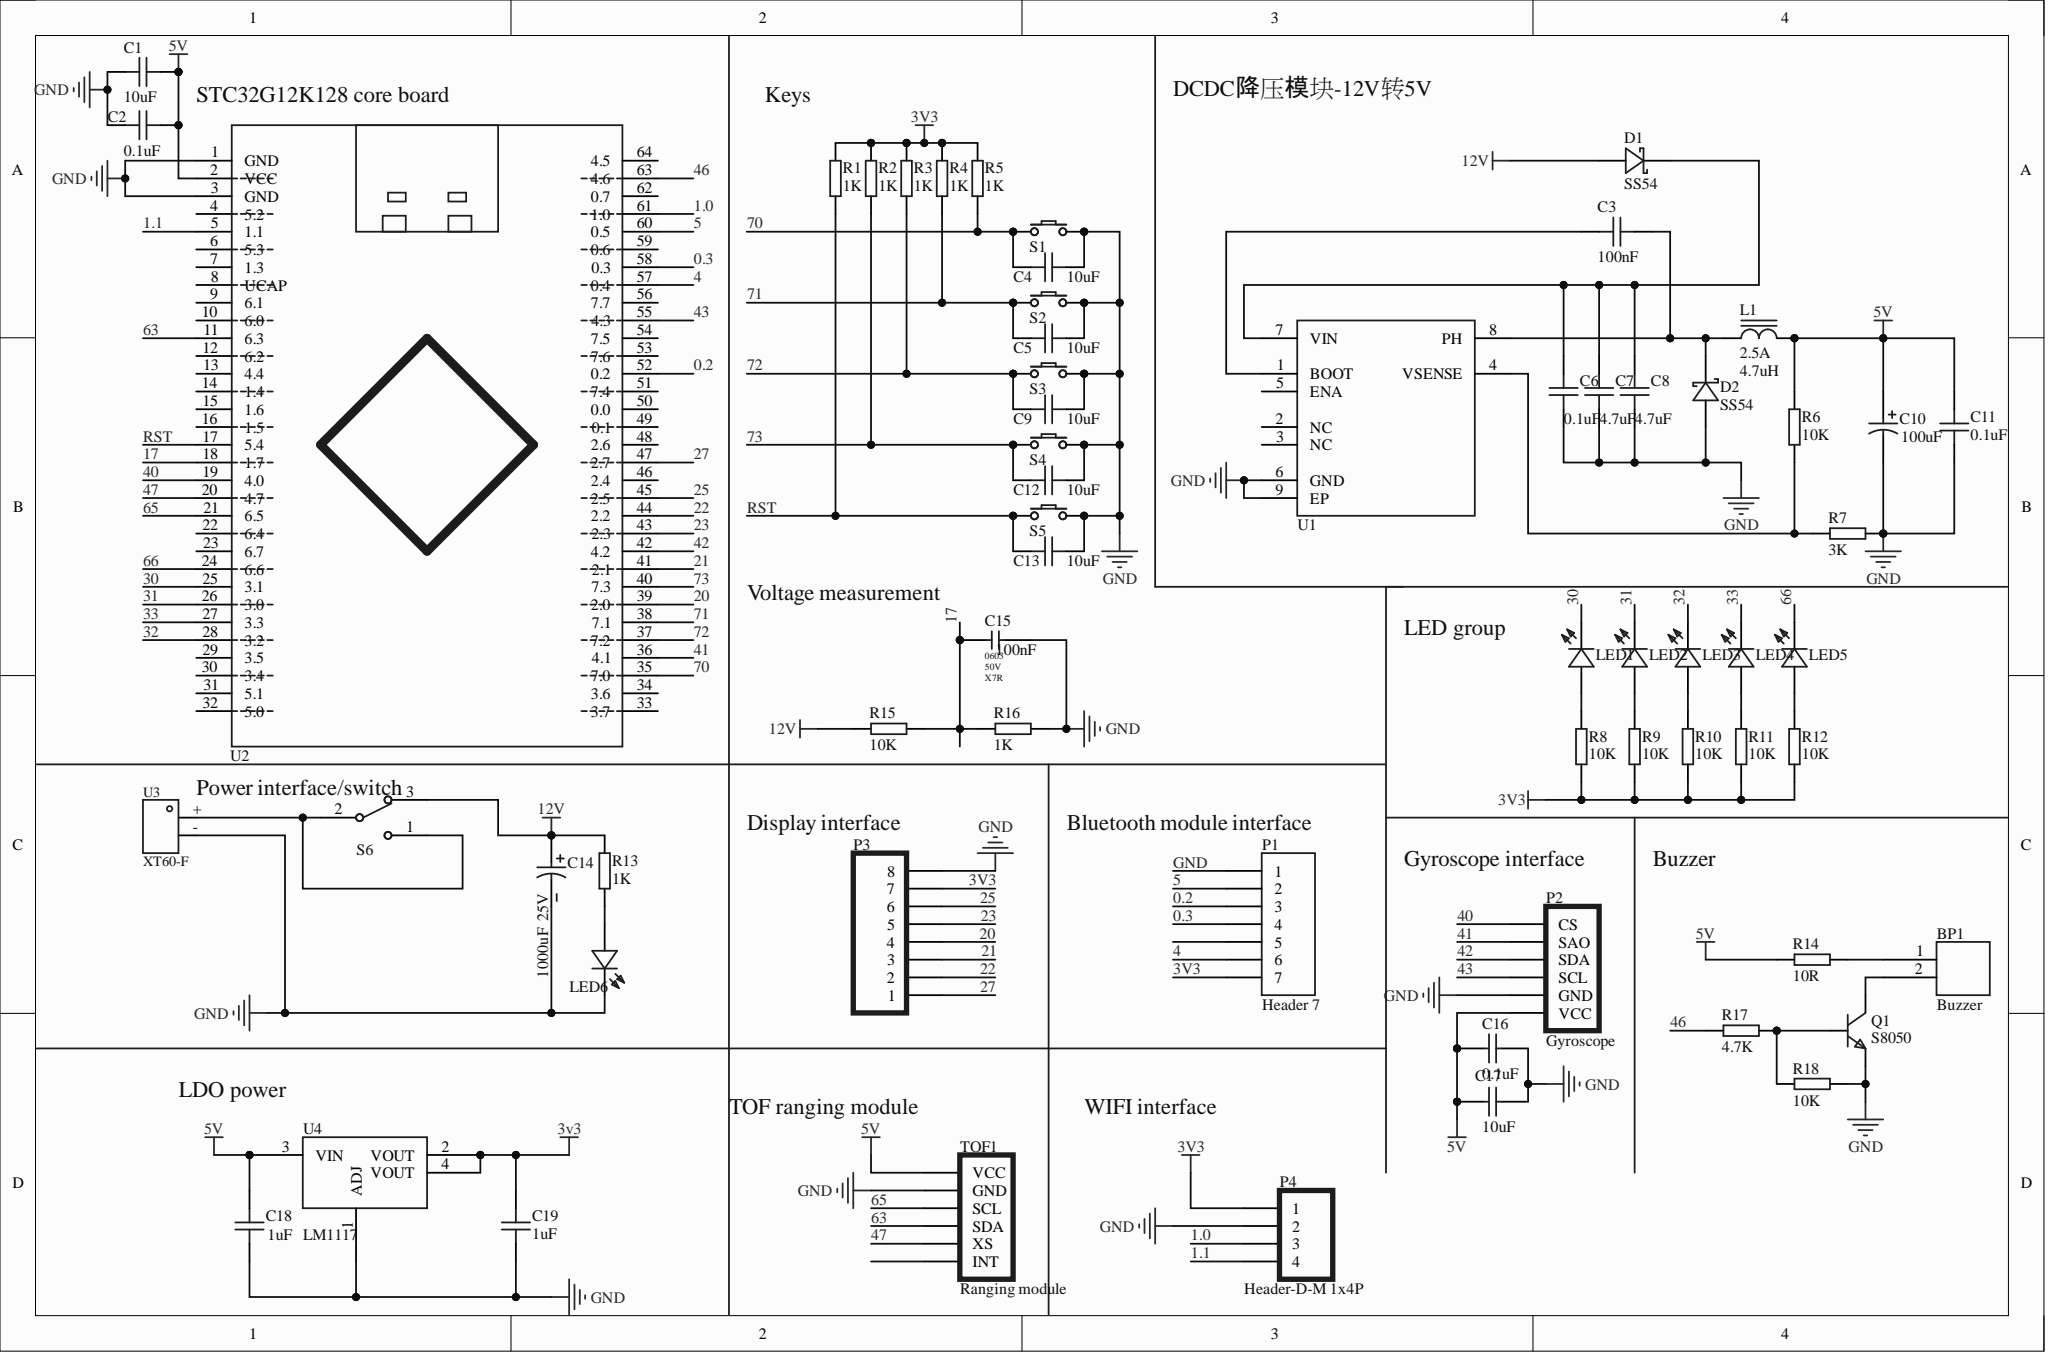Circuit board | Altium Designer | 63 parts | 49 nets
Bill of materials:
Comment,Description,Designator,Footprint,LibRef,Quantity
"Buzzer","","BP1","5*10fengmiqi","蜂鸣器","1"
"10uF","SMD capacitor","C1, C4, C5, C9, C12, C13","CAPC1608[0603]S-N","10uF","6"
"0.1uF","SMD capacitor","C2, C6, C11","CAPC1608[0603]S-N","0.1uF","3"
"100nF","SMD capacitor","C3","CAPC1608[0603]S-N","100nF","1"
"4.7uF","SMD capacitor","C7, C8","CAPC1608[0603]S-N","4.7uF","2"
"","Polarized Capacitor (Radial), SMD ceramic capacitor; MLCC; 0603(1608);, SMD capacitor","C10, C15, C16, C17","CAPC1608[0603]S-N","=Value+' '+Voltage, =Value +' '+ Voltage + ' ' + Type, =Value + ' ' + Tolerance +' '+ Voltage, =Value + ' ' + Tolerance +' '+ Voltage_1","4"
"1000uF  25V","Through-hole electrolytic capacitor","C14","CAPC1608[0603]S-N","1000uF  25V","1"
"1uF","SMD capacitor","C18, C19","CAPC1608[0603]S-N","1uF","2"
"SS54","SS54 Schottky diode","D1, D2","SOD-123-L","SS54","2"
"","Power inductor","L1","0402 TPC 4*4*2","=Value + ' ' + Imax","1"
"LED","SMD LED","LED1, LED2, LED3, LED4, LED5, LED6","LEDC1608(0603)","LED","6"
"Header 7","Header, 7-Pin","P1","HDR1X7","Header 7","1"
"Gyroscope","Header, 6-Pin","P2","HDR1X6","陀螺仪","1"
"Header  1X8","1X8","P3","HDR1X8","Header  1X8","1"
"Header-D-M 1x4P","1x4pin, through-hole, pin header","P4","HDR1X4","Header-D-M 1x4P","1"
"S8050","Discrete NPN Bipolar Transistor","Q1","SOT-23","S8050","1"
"1K","SMD resistor","R1, R2, R3, R4, R5, R13","RESC1608[0603]S-N","1K","6"
"10K","SMD resistor","R6, R8, R9, R10, R11, R12","RESC1608[0603]S-N","10K","6"
"3K","SMD resistor","R7","RESC1608[0603]S-N","3K","1"
"","SMD resistor","R14, R15, R16, R17, R18","RESC1608[0603]S-N","=Value+' '+Tolerance_2, =Value+' '+Tolerance_1, =Value+' '+Tolerance, =Value+' '+Tolerance_3","5"
"KEY","Keys","S1, S2, S3, S4, S5","anjiantiepiankaiguan","KEY","5"
"SW","SPDT switch","S6","SS12D10","SW","1"
"Ranging module","Header, 6-Pin","TOF1","HDR1X6","测距模块","1"
"TPS5450","5v regulator chip","U1","5450","TPS5450","1"
"STC32G12K128","STC32G12K128 core board","U2","STC16F40K128_CoreBoard","STC32G12K128","1"
"XT60-F","","U3","XT60","XT60-F","1"
"LM1117","3.3V regulator","U4","LM1117 - duplicate","LM1117","1"
Netlist (Protel format):
[
BP1
5*10fengmiqi
Buzzer



]
[
C1
CAPC1608[0603]S-N
10uF



]
[
C2
CAPC1608[0603]S-N
0.1uF



]
[
C3
CAPC1608[0603]S-N
100nF



]
[
C4
CAPC1608[0603]S-N
10uF



]
[
C5
CAPC1608[0603]S-N
10uF



]
[
C6
CAPC1608[0603]S-N
0.1uF



]
[
C7
CAPC1608[0603]S-N
4.7uF



]
[
C8
CAPC1608[0603]S-N
4.7uF



]
[
C9
CAPC1608[0603]S-N
10uF



]
[
C10
CAPC1608[0603]S-N




]
[
C11
CAPC1608[0603]S-N
0.1uF



]
[
C12
CAPC1608[0603]S-N
10uF



]
[
C13
CAPC1608[0603]S-N
10uF



]
[
C14
CAPC1608[0603]S-N
1000uF  25V



]
[
C15
CAPC1608[0603]S-N




]
[
C16
CAPC1608[0603]S-N




]
[
C17
CAPC1608[0603]S-N




]
[
C18
CAPC1608[0603]S-N
1uF



]
[
C19
CAPC1608[0603]S-N
1uF



]
[
D1
SOD-123-L
SS54



]
[
D2
SOD-123-L
SS54



]
[
L1
0402 TPC 4*4*2




]
[
LED1
LEDC1608(0603)
LED



]
[
LED2
LEDC1608(0603)
LED



]
[
LED3
LEDC1608(0603)
LED



]
[
LED4
LEDC1608(0603)
LED



]
[
LED5
LEDC1608(0603)
LED



]
[
LED6
LEDC1608(0603)
LED



]
[
P1
HDR1X7
Header 7



]
[
P2
HDR1X6
Gyroscope



]
[
P3
HDR1X8
Header  1X8



]
[
P4
HDR1X4
Header-D-M 1x4P



]
[
Q1
SOT-23
S8050



]
[
R1
RESC1608[0603]S-N
1K



]
[
R2
RESC1608[0603]S-N
1K



]
[
R3
RESC1608[0603]S-N
1K



]
[
R4
RESC1608[0603]S-N
1K



]
[
R5
RESC1608[0603]S-N
1K



]
[
R6
RESC1608[0603]S-N
10K



]
[
R7
RESC1608[0603]S-N
3K



]
[
R8
RESC1608[0603]S-N
10K



]
[
R9
RESC1608[0603]S-N
10K



]
[
R10
RESC1608[0603]S-N
10K



]
[
R11
RESC1608[0603]S-N
10K



]
[
R12
RESC1608[0603]S-N
10K



]
[
R13
RESC1608[0603]S-N
1K



]
[
R14
RESC1608[0603]S-N




]
[
R15
RESC1608[0603]S-N




]
[
R16
RESC1608[0603]S-N




]
[
R17
RESC1608[0603]S-N




]
[
R18
RESC1608[0603]S-N




]
[
S1
anjiantiepiankaiguan
KEY



]
[
S2
anjiantiepiankaiguan
KEY



]
[
S3
anjiantiepiankaiguan
KEY



]
[
S4
anjiantiepiankaiguan
KEY



]
[
S5
anjiantiepiankaiguan
KEY



]
[
S6
SS12D10
SW



]
[
TOF1
HDR1X6
Ranging module



]
[
U1
5450
TPS5450



]
[
U2
STC16F40K128_CoreBoard
STC32G12K128



]
[
U3
XT60
XT60-F



]
[
U4
LM1117 - duplicate
LM1117



]
(
RST
C13-1
R1-1
S5-2
U2-17
)
(
NetS6_1
S6-1
S6-2
U3-+
)
(
NetR6_1
R6-1
R7-1
U1-4
)
(
NetQ1_1
Q1-1
R17-2
R18-1
)
(
NetLED6_A
LED6-A
R13-2
)
(
NetLED5_A
LED5-A
R12-2
)
(
NetLED4_A
LED4-A
R11-2
)
(
NetLED3_A
LED3-A
R10-2
)
(
NetLED2_A
LED2-A
R9-2
)
(
NetLED1_A
LED1-A
R8-2
)
(
NetC6_2
C6-2
C7-2
C8-2
D1-K
U1-7
)
(
NetC3_2
C3-2
D2-K
L1-1
U1-8
)
(
NetC3_1
C3-1
U1-1
)
(
NetBP1_2
BP1-2
Q1-3
)
(
NetBP1_1
BP1-1
R14-2
)
(
GND
C1-1
C2-1
C4-2
C5-2
C6-1
C7-1
C8-1
C9-2
C10-2
C11-1
C12-2
C13-2
C14-2
C15-2
C16-2
C17-2
C18-1
C19-1
D2-A
LED6-C
P1-1
P2-5
P3-8
P4-2
Q1-2
R7-2
R16-2
R18-2
S1-1
S2-1
S3-1
S4-1
S5-1
TOF1-2
U1-6
U1-9
U2-1
U2-3
U3--
U4-1
)
(
73
C12-1
R2-1
S4-2
U2-40
)
(
72
C9-1
R3-1
S3-2
U2-37
)
(
71
C5-1
R4-1
S2-2
U2-38
)
(
70
C4-1
R5-1
S1-2
U2-35
)
(
66
LED5-C
U2-24
)
(
65
TOF1-3
U2-21
)
(
63
TOF1-4
U2-11
)
(
47
TOF1-5
U2-20
)
(
46
R17-1
U2-63
)
(
43
P2-4
U2-55
)
(
42
P2-3
U2-42
)
(
41
P2-2
U2-36
)
(
40
P2-1
U2-19
)
(
33
LED4-C
U2-27
)
(
32
LED3-C
U2-28
)
(
31
LED2-C
U2-26
)
(
30
LED1-C
U2-25
)
(
27
P3-1
U2-47
)
(
25
P3-6
U2-45
)
(
23
P3-5
U2-43
)
(
22
P3-2
U2-44
)
(
21
P3-3
U2-41
)
(
20
P3-4
U2-39
)
(
17
C15-1
R15-2
R16-1
U2-18
)
(
12V
C14-1
D1-A
R13-1
R15-1
S6-3
)
(
5V
C1-2
C2-2
C10-1
C11-2
C16-1
C17-1
C18-2
L1-2
P2-6
R6-2
R14-1
TOF1-1
U2-2
U4-3
)
(
5
P1-2
U2-60
)
(
4
P1-6
U2-57
)
(
3V3
C19-2
P1-7
P3-7
P4-1
R1-2
R2-2
R3-2
R4-2
R5-2
R8-1
R9-1
R10-1
R11-1
R12-1
U4-2
U4-4
)
(
1.1
P4-4
U2-5
)
(
1.0
P4-3
U2-61
)
(
0.3
P1-4
U2-58
)
(
0.2
P1-3
U2-52
)